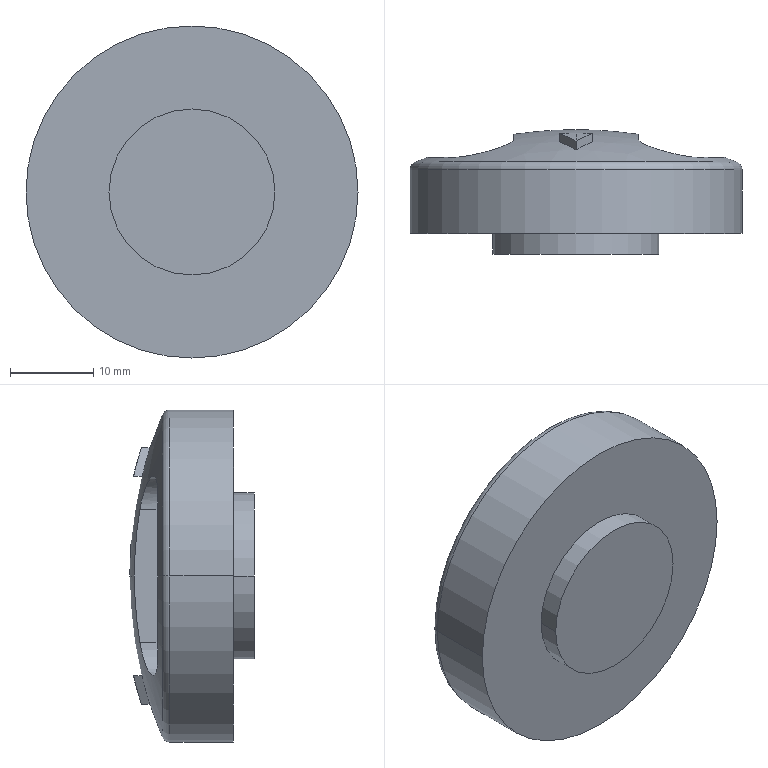Part | SolidWorks | features ICE 3, Fillet 1, RevCut 1, Revolution 1 | 1 solid | 31 faces | box 40 x 15 x 40 mm | volume 12868 mm3 | plane 12 | cylinder 11 | sphere 6 | torus 2 | commonest cylinder face diameters 7.99 x4 36 x3 20 x2 40 x2
STEP:
#1=CARTESIAN_POINT('',(-2.,12.028,-12.));
#2=VERTEX_POINT('',#1);
#3=CARTESIAN_POINT('',(0.,12.068,-12.));
#4=VERTEX_POINT('',#3);
#5=CARTESIAN_POINT('',(0.,-37.5,-12.));
#6=DIRECTION('',(0.,0.,-1.));
#7=DIRECTION('',(1.,0.,0.));
#8=AXIS2_PLACEMENT_3D('',#5,#6,#7);
#9=CIRCLE('',#8,49.568);
#10=EDGE_CURVE('',#2,#4,#9,.T.);
#11=ORIENTED_EDGE('',*,*,#10,.T.);
#12=CARTESIAN_POINT('',(0.,11.099,-15.464));
#13=VERTEX_POINT('',#12);
#14=CARTESIAN_POINT('',(0.,-37.5,0.));
#15=DIRECTION('',(-1.,0.,0.));
#16=DIRECTION('',(0.,0.,1.));
#17=AXIS2_PLACEMENT_3D('',#14,#15,#16);
#18=CIRCLE('',#17,51.);
#19=EDGE_CURVE('',#4,#13,#18,.T.);
#20=ORIENTED_EDGE('',*,*,#19,.T.);
#21=CARTESIAN_POINT('',(-6.696,-37.5,-3.866));
#22=DIRECTION('',(0.866,0.,0.5));
#23=DIRECTION('',(-0.5,0.,0.866));
#24=AXIS2_PLACEMENT_3D('',#21,#22,#23);
#25=CIRCLE('',#24,50.41);
#26=EDGE_CURVE('',#13,#2,#25,.T.);
#27=ORIENTED_EDGE('',*,*,#26,.T.);
#28=EDGE_LOOP('',(#11,#20,#27));
#29=FACE_OUTER_BOUND('',#28,.T.);
#30=CARTESIAN_POINT('',(0.,-37.5,0.));
#31=DIRECTION('',(1.,0.,0.));
#32=DIRECTION('',(0.,0.,-1.));
#33=AXIS2_PLACEMENT_3D('',#30,#31,#32);
#34=SPHERICAL_SURFACE('',#33,51.);
#35=ADVANCED_FACE('',(#29),#34,.T.);
#36=CARTESIAN_POINT('',(2.,12.028,12.));
#37=VERTEX_POINT('',#36);
#38=CARTESIAN_POINT('',(0.,12.068,12.));
#39=VERTEX_POINT('',#38);
#40=CARTESIAN_POINT('',(0.,-37.5,12.));
#41=DIRECTION('',(0.,0.,1.));
#42=DIRECTION('',(-1.,0.,0.));
#43=AXIS2_PLACEMENT_3D('',#40,#41,#42);
#44=CIRCLE('',#43,49.568);
#45=EDGE_CURVE('',#37,#39,#44,.T.);
#46=ORIENTED_EDGE('',*,*,#45,.T.);
#47=CARTESIAN_POINT('',(0.,11.099,15.464));
#48=VERTEX_POINT('',#47);
#49=CARTESIAN_POINT('',(0.,-37.5,0.));
#50=DIRECTION('',(1.,0.,0.));
#51=DIRECTION('',(0.,0.,-1.));
#52=AXIS2_PLACEMENT_3D('',#49,#50,#51);
#53=CIRCLE('',#52,51.);
#54=EDGE_CURVE('',#39,#48,#53,.T.);
#55=ORIENTED_EDGE('',*,*,#54,.T.);
#56=CARTESIAN_POINT('',(6.696,-37.5,3.866));
#57=DIRECTION('',(-0.866,0.,-0.5));
#58=DIRECTION('',(0.5,0.,-0.866));
#59=AXIS2_PLACEMENT_3D('',#56,#57,#58);
#60=CIRCLE('',#59,50.41);
#61=EDGE_CURVE('',#48,#37,#60,.T.);
#62=ORIENTED_EDGE('',*,*,#61,.T.);
#63=EDGE_LOOP('',(#46,#55,#62));
#64=FACE_OUTER_BOUND('',#63,.T.);
#65=CARTESIAN_POINT('',(0.,-37.5,0.));
#66=DIRECTION('',(1.,0.,0.));
#67=DIRECTION('',(0.,0.,-1.));
#68=AXIS2_PLACEMENT_3D('',#65,#66,#67);
#69=SPHERICAL_SURFACE('',#68,51.);
#70=ADVANCED_FACE('',(#64),#69,.T.);
#71=CARTESIAN_POINT('',(14.774,9.148,10.282));
#72=VERTEX_POINT('',#71);
#73=CARTESIAN_POINT('',(18.,9.148,0.));
#74=VERTEX_POINT('',#73);
#75=CARTESIAN_POINT('',(0.,9.148,0.));
#76=DIRECTION('',(0.,1.,0.));
#77=DIRECTION('',(1.,0.,0.));
#78=AXIS2_PLACEMENT_3D('',#75,#76,#77);
#79=CIRCLE('',#78,18.);
#80=EDGE_CURVE('',#72,#74,#79,.T.);
#81=ORIENTED_EDGE('',*,*,#80,.T.);
#82=CARTESIAN_POINT('',(18.,8.,0.));
#83=VERTEX_POINT('',#82);
#84=CARTESIAN_POINT('',(18.,18.5,0.));
#85=DIRECTION('',(0.,-1.,0.));
#86=VECTOR('',#85,1000.);
#87=LINE('',#84,#86);
#88=EDGE_CURVE('',#74,#83,#87,.T.);
#89=ORIENTED_EDGE('',*,*,#88,.T.);
#90=CARTESIAN_POINT('',(14.774,8.,10.282));
#91=VERTEX_POINT('',#90);
#92=CARTESIAN_POINT('',(0.,8.,0.));
#93=DIRECTION('',(0.,-1.,0.));
#94=DIRECTION('',(-1.,0.,0.));
#95=AXIS2_PLACEMENT_3D('',#92,#93,#94);
#96=CIRCLE('',#95,18.);
#97=EDGE_CURVE('',#83,#91,#96,.T.);
#98=ORIENTED_EDGE('',*,*,#97,.T.);
#99=CARTESIAN_POINT('',(14.774,18.5,10.282));
#100=DIRECTION('',(0.,-1.,0.));
#101=VECTOR('',#100,1000.);
#102=LINE('',#99,#101);
#103=EDGE_CURVE('',#72,#91,#102,.T.);
#104=ORIENTED_EDGE('',*,*,#103,.F.);
#105=EDGE_LOOP('',(#81,#89,#98,#104));
#106=FACE_OUTER_BOUND('',#105,.T.);
#107=CARTESIAN_POINT('',(0.,18.5,0.));
#108=DIRECTION('',(0.,-1.,0.));
#109=DIRECTION('',(1.,0.,0.));
#110=AXIS2_PLACEMENT_3D('',#107,#108,#109);
#111=CYLINDRICAL_SURFACE('',#110,18.);
#112=ADVANCED_FACE('',(#106),#111,.F.);
#113=CARTESIAN_POINT('',(10.,-2.5,0.));
#114=VERTEX_POINT('',#113);
#115=CARTESIAN_POINT('',(-10.,-2.5,0.));
#116=VERTEX_POINT('',#115);
#117=CARTESIAN_POINT('',(0.,-2.5,0.));
#118=DIRECTION('',(0.,-1.,0.));
#119=DIRECTION('',(1.,0.,0.));
#120=AXIS2_PLACEMENT_3D('',#117,#118,#119);
#121=CIRCLE('',#120,10.);
#122=EDGE_CURVE('',#114,#116,#121,.T.);
#123=ORIENTED_EDGE('',*,*,#122,.F.);
#124=CARTESIAN_POINT('',(10.,0.,0.));
#125=VERTEX_POINT('',#124);
#126=CARTESIAN_POINT('',(10.,-2.5,0.));
#127=DIRECTION('',(0.,1.,0.));
#128=VECTOR('',#127,1000.);
#129=LINE('',#126,#128);
#130=EDGE_CURVE('',#114,#125,#129,.T.);
#131=ORIENTED_EDGE('',*,*,#130,.T.);
#132=CARTESIAN_POINT('',(-10.,0.,0.));
#133=VERTEX_POINT('',#132);
#134=CARTESIAN_POINT('',(0.,0.,0.));
#135=DIRECTION('',(0.,-1.,0.));
#136=DIRECTION('',(1.,0.,0.));
#137=AXIS2_PLACEMENT_3D('',#134,#135,#136);
#138=CIRCLE('',#137,10.);
#139=EDGE_CURVE('',#125,#133,#138,.T.);
#140=ORIENTED_EDGE('',*,*,#139,.T.);
#141=CARTESIAN_POINT('',(-10.,-2.5,0.));
#142=DIRECTION('',(0.,1.,0.));
#143=VECTOR('',#142,1000.);
#144=LINE('',#141,#143);
#145=EDGE_CURVE('',#116,#133,#144,.T.);
#146=ORIENTED_EDGE('',*,*,#145,.F.);
#147=EDGE_LOOP('',(#123,#131,#140,#146));
#148=FACE_OUTER_BOUND('',#147,.T.);
#149=CARTESIAN_POINT('',(0.,-2.5,0.));
#150=DIRECTION('',(0.,1.,0.));
#151=DIRECTION('',(-1.,0.,0.));
#152=AXIS2_PLACEMENT_3D('',#149,#150,#151);
#153=CYLINDRICAL_SURFACE('',#152,10.);
#154=ADVANCED_FACE('',(#148),#153,.T.);
#155=CARTESIAN_POINT('',(-19.388,8.588,0.));
#156=VERTEX_POINT('',#155);
#157=CARTESIAN_POINT('',(19.388,8.588,0.));
#158=VERTEX_POINT('',#157);
#159=CARTESIAN_POINT('',(0.,8.588,0.));
#160=DIRECTION('',(0.,1.,0.));
#161=DIRECTION('',(1.,0.,0.));
#162=AXIS2_PLACEMENT_3D('',#159,#160,#161);
#163=CIRCLE('',#162,19.388);
#164=EDGE_CURVE('',#156,#158,#163,.T.);
#165=ORIENTED_EDGE('',*,*,#164,.F.);
#166=CARTESIAN_POINT('',(-20.,7.666,0.));
#167=VERTEX_POINT('',#166);
#168=CARTESIAN_POINT('',(-19.,7.666,0.));
#169=DIRECTION('',(0.,0.,1.));
#170=DIRECTION('',(1.,0.,0.));
#171=AXIS2_PLACEMENT_3D('',#168,#169,#170);
#172=CIRCLE('',#171,1.);
#173=EDGE_CURVE('',#156,#167,#172,.T.);
#174=ORIENTED_EDGE('',*,*,#173,.T.);
#175=CARTESIAN_POINT('',(20.,7.666,0.));
#176=VERTEX_POINT('',#175);
#177=CARTESIAN_POINT('',(0.,7.666,0.));
#178=DIRECTION('',(0.,-1.,0.));
#179=DIRECTION('',(1.,0.,0.));
#180=AXIS2_PLACEMENT_3D('',#177,#178,#179);
#181=CIRCLE('',#180,20.);
#182=EDGE_CURVE('',#176,#167,#181,.T.);
#183=ORIENTED_EDGE('',*,*,#182,.F.);
#184=CARTESIAN_POINT('',(19.,7.666,0.));
#185=DIRECTION('',(0.,0.,-1.));
#186=DIRECTION('',(-1.,0.,0.));
#187=AXIS2_PLACEMENT_3D('',#184,#185,#186);
#188=CIRCLE('',#187,1.);
#189=EDGE_CURVE('',#158,#176,#188,.T.);
#190=ORIENTED_EDGE('',*,*,#189,.F.);
#191=EDGE_LOOP('',(#165,#174,#183,#190));
#192=FACE_OUTER_BOUND('',#191,.T.);
#193=CARTESIAN_POINT('',(0.,7.666,0.));
#194=DIRECTION('',(0.,-1.,0.));
#195=DIRECTION('',(1.,0.,0.));
#196=AXIS2_PLACEMENT_3D('',#193,#194,#195);
#197=TOROIDAL_SURFACE('',#196,19.,1.);
#198=ADVANCED_FACE('',(#192),#197,.T.);
#199=ORIENTED_EDGE('',*,*,#182,.T.);
#200=CARTESIAN_POINT('',(-20.,0.,0.));
#201=VERTEX_POINT('',#200);
#202=CARTESIAN_POINT('',(-20.,0.,0.));
#203=DIRECTION('',(0.,-1.,0.));
#204=VECTOR('',#203,1000.);
#205=LINE('',#202,#204);
#206=EDGE_CURVE('',#167,#201,#205,.T.);
#207=ORIENTED_EDGE('',*,*,#206,.T.);
#208=CARTESIAN_POINT('',(20.,0.,0.));
#209=VERTEX_POINT('',#208);
#210=CARTESIAN_POINT('',(0.,0.,0.));
#211=DIRECTION('',(0.,-1.,0.));
#212=DIRECTION('',(1.,0.,0.));
#213=AXIS2_PLACEMENT_3D('',#210,#211,#212);
#214=CIRCLE('',#213,20.);
#215=EDGE_CURVE('',#209,#201,#214,.T.);
#216=ORIENTED_EDGE('',*,*,#215,.F.);
#217=CARTESIAN_POINT('',(20.,0.,0.));
#218=DIRECTION('',(0.,-1.,0.));
#219=VECTOR('',#218,1000.);
#220=LINE('',#217,#219);
#221=EDGE_CURVE('',#176,#209,#220,.T.);
#222=ORIENTED_EDGE('',*,*,#221,.F.);
#223=EDGE_LOOP('',(#199,#207,#216,#222));
#224=FACE_OUTER_BOUND('',#223,.T.);
#225=CARTESIAN_POINT('',(0.,0.,0.));
#226=DIRECTION('',(0.,-1.,0.));
#227=DIRECTION('',(1.,0.,0.));
#228=AXIS2_PLACEMENT_3D('',#225,#226,#227);
#229=CYLINDRICAL_SURFACE('',#228,20.);
#230=ADVANCED_FACE('',(#224),#229,.T.);
#231=CARTESIAN_POINT('',(2.,10.997,12.));
#232=VERTEX_POINT('',#231);
#233=CARTESIAN_POINT('',(-2.,10.997,12.));
#234=VERTEX_POINT('',#233);
#235=CARTESIAN_POINT('',(0.,-37.5,12.));
#236=DIRECTION('',(0.,0.,1.));
#237=DIRECTION('',(-1.,0.,0.));
#238=AXIS2_PLACEMENT_3D('',#235,#236,#237);
#239=CIRCLE('',#238,48.539);
#240=EDGE_CURVE('',#232,#234,#239,.T.);
#241=ORIENTED_EDGE('',*,*,#240,.F.);
#242=CARTESIAN_POINT('',(0.,10.049,15.464));
#243=VERTEX_POINT('',#242);
#244=CARTESIAN_POINT('',(6.696,-37.5,3.866));
#245=DIRECTION('',(-0.866,0.,-0.5));
#246=DIRECTION('',(0.5,0.,-0.866));
#247=AXIS2_PLACEMENT_3D('',#244,#245,#246);
#248=CIRCLE('',#247,49.399);
#249=EDGE_CURVE('',#243,#232,#248,.T.);
#250=ORIENTED_EDGE('',*,*,#249,.F.);
#251=CARTESIAN_POINT('',(-6.696,-37.5,3.866));
#252=DIRECTION('',(0.866,0.,-0.5));
#253=DIRECTION('',(0.5,0.,0.866));
#254=AXIS2_PLACEMENT_3D('',#251,#252,#253);
#255=CIRCLE('',#254,49.399);
#256=EDGE_CURVE('',#234,#243,#255,.T.);
#257=ORIENTED_EDGE('',*,*,#256,.F.);
#258=EDGE_LOOP('',(#241,#250,#257));
#259=FACE_BOUND('',#258,.T.);
#260=CARTESIAN_POINT('',(0.,12.5,0.));
#261=VERTEX_POINT('',#260);
#262=CARTESIAN_POINT('',(7.5,11.934,0.));
#263=VERTEX_POINT('',#262);
#264=CARTESIAN_POINT('',(0.,-37.5,0.));
#265=DIRECTION('',(0.,0.,-1.));
#266=DIRECTION('',(-1.,0.,0.));
#267=AXIS2_PLACEMENT_3D('',#264,#265,#266);
#268=CIRCLE('',#267,50.);
#269=EDGE_CURVE('',#261,#263,#268,.T.);
#270=ORIENTED_EDGE('',*,*,#269,.F.);
#271=CARTESIAN_POINT('',(-7.5,11.934,0.));
#272=VERTEX_POINT('',#271);
#273=CARTESIAN_POINT('',(0.,-37.5,0.));
#274=DIRECTION('',(0.,0.,1.));
#275=DIRECTION('',(1.,0.,0.));
#276=AXIS2_PLACEMENT_3D('',#273,#274,#275);
#277=CIRCLE('',#276,50.);
#278=EDGE_CURVE('',#261,#272,#277,.T.);
#279=ORIENTED_EDGE('',*,*,#278,.T.);
#280=CARTESIAN_POINT('',(-7.5,11.283,8.));
#281=VERTEX_POINT('',#280);
#282=CARTESIAN_POINT('',(-7.5,-37.5,0.));
#283=DIRECTION('',(-1.,0.,0.));
#284=DIRECTION('',(0.,0.,-1.));
#285=AXIS2_PLACEMENT_3D('',#282,#283,#284);
#286=CIRCLE('',#285,49.434);
#287=EDGE_CURVE('',#281,#272,#286,.T.);
#288=ORIENTED_EDGE('',*,*,#287,.F.);
#289=CARTESIAN_POINT('',(-14.774,9.148,10.282));
#290=VERTEX_POINT('',#289);
#291=CARTESIAN_POINT('',(-14.774,9.148,10.282));
#292=CARTESIAN_POINT('',(-14.525,9.148,10.64));
#293=CARTESIAN_POINT('',(-14.226,9.169,10.949));
#294=CARTESIAN_POINT('',(-13.528,9.251,11.466));
#295=CARTESIAN_POINT('',(-13.149,9.311,11.662));
#296=CARTESIAN_POINT('',(-12.334,9.465,11.93));
#297=CARTESIAN_POINT('',(-11.917,9.556,11.995));
#298=CARTESIAN_POINT('',(-11.071,9.762,11.995));
#299=CARTESIAN_POINT('',(-10.659,9.874,11.929));
#300=CARTESIAN_POINT('',(-10.063,10.051,11.736));
#301=CARTESIAN_POINT('',(-9.87,10.111,11.655));
#302=CARTESIAN_POINT('',(-9.501,10.231,11.468));
#303=CARTESIAN_POINT('',(-9.325,10.292,11.361));
#304=CARTESIAN_POINT('',(-8.988,10.413,11.118));
#305=CARTESIAN_POINT('',(-8.828,10.474,10.982));
#306=CARTESIAN_POINT('',(-8.534,10.593,10.69));
#307=CARTESIAN_POINT('',(-8.399,10.651,10.533));
#308=CARTESIAN_POINT('',(-8.153,10.766,10.198));
#309=CARTESIAN_POINT('',(-8.041,10.822,10.019));
#310=CARTESIAN_POINT('',(-7.849,10.929,9.646));
#311=CARTESIAN_POINT('',(-7.768,10.98,9.453));
#312=CARTESIAN_POINT('',(-7.571,11.125,8.857));
#313=CARTESIAN_POINT('',(-7.5,11.212,8.431));
#314=CARTESIAN_POINT('',(-7.5,11.283,8.));
#315=B_SPLINE_CURVE_WITH_KNOTS('',3,(#291,#292,#293,#294,#295,#296,#297,#298,#299,#300,#301,#302,#303,#304,#305,#306,#307,#308,#309,#310,#311,#312,#313,#314),.UNSPECIFIED.,.F.,.F.,(4,2,2,2,2,2,2,2,2,2,2,4),(0.000000345,0.001291,0.002581,0.003872,0.005162,0.005808,0.006453,0.007098,0.007744,0.008389,0.009034,0.01032),.UNSPECIFIED.);
#316=EDGE_CURVE('',#290,#281,#315,.T.);
#317=ORIENTED_EDGE('',*,*,#316,.F.);
#318=CARTESIAN_POINT('',(-18.,9.148,0.));
#319=VERTEX_POINT('',#318);
#320=CARTESIAN_POINT('',(0.,9.148,0.));
#321=DIRECTION('',(0.,1.,0.));
#322=DIRECTION('',(1.,0.,0.));
#323=AXIS2_PLACEMENT_3D('',#320,#321,#322);
#324=CIRCLE('',#323,18.);
#325=EDGE_CURVE('',#319,#290,#324,.T.);
#326=ORIENTED_EDGE('',*,*,#325,.F.);
#327=CARTESIAN_POINT('',(0.,-37.5,0.));
#328=DIRECTION('',(0.,0.,1.));
#329=DIRECTION('',(1.,0.,0.));
#330=AXIS2_PLACEMENT_3D('',#327,#328,#329);
#331=CIRCLE('',#330,50.);
#332=EDGE_CURVE('',#319,#156,#331,.T.);
#333=ORIENTED_EDGE('',*,*,#332,.T.);
#334=ORIENTED_EDGE('',*,*,#164,.T.);
#335=CARTESIAN_POINT('',(0.,-37.5,0.));
#336=DIRECTION('',(0.,0.,-1.));
#337=DIRECTION('',(-1.,0.,0.));
#338=AXIS2_PLACEMENT_3D('',#335,#336,#337);
#339=CIRCLE('',#338,50.);
#340=EDGE_CURVE('',#74,#158,#339,.T.);
#341=ORIENTED_EDGE('',*,*,#340,.F.);
#342=ORIENTED_EDGE('',*,*,#80,.F.);
#343=CARTESIAN_POINT('',(7.5,11.283,8.));
#344=VERTEX_POINT('',#343);
#345=CARTESIAN_POINT('',(7.5,11.283,8.));
#346=CARTESIAN_POINT('',(7.5,11.212,8.431));
#347=CARTESIAN_POINT('',(7.568,11.128,8.847));
#348=CARTESIAN_POINT('',(7.767,10.981,9.451));
#349=CARTESIAN_POINT('',(7.849,10.929,9.646));
#350=CARTESIAN_POINT('',(8.04,10.823,10.016));
#351=CARTESIAN_POINT('',(8.149,10.767,10.193));
#352=CARTESIAN_POINT('',(8.397,10.652,10.531));
#353=CARTESIAN_POINT('',(8.534,10.593,10.69));
#354=CARTESIAN_POINT('',(8.828,10.474,10.982));
#355=CARTESIAN_POINT('',(8.986,10.414,11.116));
#356=CARTESIAN_POINT('',(9.322,10.293,11.359));
#357=CARTESIAN_POINT('',(9.501,10.231,11.468));
#358=CARTESIAN_POINT('',(9.871,10.11,11.656));
#359=CARTESIAN_POINT('',(10.062,10.051,11.735));
#360=CARTESIAN_POINT('',(10.456,9.934,11.863));
#361=CARTESIAN_POINT('',(10.661,9.876,11.913));
#362=CARTESIAN_POINT('',(11.075,9.764,11.978));
#363=CARTESIAN_POINT('',(11.283,9.711,11.995));
#364=CARTESIAN_POINT('',(11.909,9.558,11.995));
#365=CARTESIAN_POINT('',(12.336,9.465,11.928));
#366=CARTESIAN_POINT('',(12.939,9.351,11.731));
#367=CARTESIAN_POINT('',(13.136,9.317,11.649));
#368=CARTESIAN_POINT('',(13.518,9.256,11.452));
#369=CARTESIAN_POINT('',(13.702,9.231,11.337));
#370=CARTESIAN_POINT('',(14.046,9.19,11.082));
#371=CARTESIAN_POINT('',(14.208,9.174,10.941));
#372=CARTESIAN_POINT('',(14.51,9.153,10.63));
#373=CARTESIAN_POINT('',(14.65,9.148,10.461));
#374=CARTESIAN_POINT('',(14.774,9.148,10.282));
#375=B_SPLINE_CURVE_WITH_KNOTS('',3,(#345,#346,#347,#348,#349,#350,#351,#352,#353,#354,#355,#356,#357,#358,#359,#360,#361,#362,#363,#364,#365,#366,#367,#368,#369,#370,#371,#372,#373,#374),.UNSPECIFIED.,.F.,.F.,(4,2,2,2,2,2,2,2,2,2,2,2,2,2,4),(0.0000002,0.001291,0.001936,0.002581,0.003226,0.003871,0.004516,0.005161,0.005807,0.006452,0.007742,0.008387,0.009032,0.009678,0.01032),.UNSPECIFIED.);
#376=EDGE_CURVE('',#344,#72,#375,.T.);
#377=ORIENTED_EDGE('',*,*,#376,.F.);
#378=CARTESIAN_POINT('',(7.5,-37.5,0.));
#379=DIRECTION('',(1.,0.,0.));
#380=DIRECTION('',(0.,0.,1.));
#381=AXIS2_PLACEMENT_3D('',#378,#379,#380);
#382=CIRCLE('',#381,49.434);
#383=EDGE_CURVE('',#263,#344,#382,.T.);
#384=ORIENTED_EDGE('',*,*,#383,.F.);
#385=EDGE_LOOP('',(#270,#279,#288,#317,#326,#333,#334,#341,#342,#377,#384));
#386=FACE_OUTER_BOUND('',#385,.T.);
#387=CARTESIAN_POINT('',(0.,-37.5,0.));
#388=DIRECTION('',(0.,0.,1.));
#389=DIRECTION('',(1.,0.,0.));
#390=AXIS2_PLACEMENT_3D('',#387,#388,#389);
#391=SPHERICAL_SURFACE('',#390,50.);
#392=ADVANCED_FACE('',(#259,#386),#391,.T.);
#393=ORIENTED_EDGE('',*,*,#10,.F.);
#394=CARTESIAN_POINT('',(-2.,10.997,-12.));
#395=VERTEX_POINT('',#394);
#396=CARTESIAN_POINT('',(-2.,13.5,-12.));
#397=DIRECTION('',(0.,-1.,0.));
#398=VECTOR('',#397,1000.);
#399=LINE('',#396,#398);
#400=EDGE_CURVE('',#2,#395,#399,.T.);
#401=ORIENTED_EDGE('',*,*,#400,.T.);
#402=CARTESIAN_POINT('',(2.,10.997,-12.));
#403=VERTEX_POINT('',#402);
#404=CARTESIAN_POINT('',(0.,-37.5,-12.));
#405=DIRECTION('',(0.,0.,-1.));
#406=DIRECTION('',(1.,0.,0.));
#407=AXIS2_PLACEMENT_3D('',#404,#405,#406);
#408=CIRCLE('',#407,48.539);
#409=EDGE_CURVE('',#395,#403,#408,.T.);
#410=ORIENTED_EDGE('',*,*,#409,.T.);
#411=CARTESIAN_POINT('',(2.,12.028,-12.));
#412=VERTEX_POINT('',#411);
#413=CARTESIAN_POINT('',(2.,13.5,-12.));
#414=DIRECTION('',(0.,-1.,0.));
#415=VECTOR('',#414,1000.);
#416=LINE('',#413,#415);
#417=EDGE_CURVE('',#412,#403,#416,.T.);
#418=ORIENTED_EDGE('',*,*,#417,.F.);
#419=CARTESIAN_POINT('',(0.,-37.5,-12.));
#420=DIRECTION('',(0.,0.,-1.));
#421=DIRECTION('',(1.,0.,0.));
#422=AXIS2_PLACEMENT_3D('',#419,#420,#421);
#423=CIRCLE('',#422,49.568);
#424=EDGE_CURVE('',#4,#412,#423,.T.);
#425=ORIENTED_EDGE('',*,*,#424,.F.);
#426=EDGE_LOOP('',(#393,#401,#410,#418,#425));
#427=FACE_OUTER_BOUND('',#426,.T.);
#428=CARTESIAN_POINT('',(-2.,13.5,-12.));
#429=DIRECTION('',(0.,0.,1.));
#430=DIRECTION('',(1.,0.,0.));
#431=AXIS2_PLACEMENT_3D('',#428,#429,#430);
#432=PLANE('',#431);
#433=ADVANCED_FACE('',(#427),#432,.T.);
#434=CARTESIAN_POINT('',(6.696,-37.5,-3.866));
#435=DIRECTION('',(-0.866,0.,0.5));
#436=DIRECTION('',(-0.5,0.,-0.866));
#437=AXIS2_PLACEMENT_3D('',#434,#435,#436);
#438=CIRCLE('',#437,50.41);
#439=EDGE_CURVE('',#412,#13,#438,.T.);
#440=ORIENTED_EDGE('',*,*,#439,.F.);
#441=ORIENTED_EDGE('',*,*,#417,.T.);
#442=CARTESIAN_POINT('',(0.,10.049,-15.464));
#443=VERTEX_POINT('',#442);
#444=CARTESIAN_POINT('',(6.696,-37.5,-3.866));
#445=DIRECTION('',(-0.866,0.,0.5));
#446=DIRECTION('',(-0.5,0.,-0.866));
#447=AXIS2_PLACEMENT_3D('',#444,#445,#446);
#448=CIRCLE('',#447,49.399);
#449=EDGE_CURVE('',#403,#443,#448,.T.);
#450=ORIENTED_EDGE('',*,*,#449,.T.);
#451=CARTESIAN_POINT('',(0.,13.5,-15.464));
#452=DIRECTION('',(0.,-1.,0.));
#453=VECTOR('',#452,1000.);
#454=LINE('',#451,#453);
#455=EDGE_CURVE('',#13,#443,#454,.T.);
#456=ORIENTED_EDGE('',*,*,#455,.F.);
#457=EDGE_LOOP('',(#440,#441,#450,#456));
#458=FACE_OUTER_BOUND('',#457,.T.);
#459=CARTESIAN_POINT('',(2.,13.5,-12.));
#460=DIRECTION('',(0.866,0.,-0.5));
#461=DIRECTION('',(-0.5,0.,-0.866));
#462=AXIS2_PLACEMENT_3D('',#459,#460,#461);
#463=PLANE('',#462);
#464=ADVANCED_FACE('',(#458),#463,.T.);
#465=ORIENTED_EDGE('',*,*,#26,.F.);
#466=ORIENTED_EDGE('',*,*,#455,.T.);
#467=CARTESIAN_POINT('',(-6.696,-37.5,-3.866));
#468=DIRECTION('',(0.866,0.,0.5));
#469=DIRECTION('',(-0.5,0.,0.866));
#470=AXIS2_PLACEMENT_3D('',#467,#468,#469);
#471=CIRCLE('',#470,49.399);
#472=EDGE_CURVE('',#443,#395,#471,.T.);
#473=ORIENTED_EDGE('',*,*,#472,.T.);
#474=ORIENTED_EDGE('',*,*,#400,.F.);
#475=EDGE_LOOP('',(#465,#466,#473,#474));
#476=FACE_OUTER_BOUND('',#475,.T.);
#477=CARTESIAN_POINT('',(0.,13.5,-15.464));
#478=DIRECTION('',(-0.866,0.,-0.5));
#479=DIRECTION('',(-0.5,0.,0.866));
#480=AXIS2_PLACEMENT_3D('',#477,#478,#479);
#481=PLANE('',#480);
#482=ADVANCED_FACE('',(#476),#481,.T.);
#483=ORIENTED_EDGE('',*,*,#45,.F.);
#484=CARTESIAN_POINT('',(2.,13.5,12.));
#485=DIRECTION('',(0.,-1.,0.));
#486=VECTOR('',#485,1000.);
#487=LINE('',#484,#486);
#488=EDGE_CURVE('',#37,#232,#487,.T.);
#489=ORIENTED_EDGE('',*,*,#488,.T.);
#490=ORIENTED_EDGE('',*,*,#240,.T.);
#491=CARTESIAN_POINT('',(-2.,12.028,12.));
#492=VERTEX_POINT('',#491);
#493=CARTESIAN_POINT('',(-2.,13.5,12.));
#494=DIRECTION('',(0.,-1.,0.));
#495=VECTOR('',#494,1000.);
#496=LINE('',#493,#495);
#497=EDGE_CURVE('',#492,#234,#496,.T.);
#498=ORIENTED_EDGE('',*,*,#497,.F.);
#499=CARTESIAN_POINT('',(0.,-37.5,12.));
#500=DIRECTION('',(0.,0.,1.));
#501=DIRECTION('',(-1.,0.,0.));
#502=AXIS2_PLACEMENT_3D('',#499,#500,#501);
#503=CIRCLE('',#502,49.568);
#504=EDGE_CURVE('',#39,#492,#503,.T.);
#505=ORIENTED_EDGE('',*,*,#504,.F.);
#506=EDGE_LOOP('',(#483,#489,#490,#498,#505));
#507=FACE_OUTER_BOUND('',#506,.T.);
#508=CARTESIAN_POINT('',(-2.,13.5,12.));
#509=DIRECTION('',(0.,0.,-1.));
#510=DIRECTION('',(-1.,0.,0.));
#511=AXIS2_PLACEMENT_3D('',#508,#509,#510);
#512=PLANE('',#511);
#513=ADVANCED_FACE('',(#507),#512,.T.);
#514=CARTESIAN_POINT('',(-6.696,-37.5,3.866));
#515=DIRECTION('',(0.866,0.,-0.5));
#516=DIRECTION('',(0.5,0.,0.866));
#517=AXIS2_PLACEMENT_3D('',#514,#515,#516);
#518=CIRCLE('',#517,50.41);
#519=EDGE_CURVE('',#492,#48,#518,.T.);
#520=ORIENTED_EDGE('',*,*,#519,.F.);
#521=ORIENTED_EDGE('',*,*,#497,.T.);
#522=ORIENTED_EDGE('',*,*,#256,.T.);
#523=CARTESIAN_POINT('',(0.,13.5,15.464));
#524=DIRECTION('',(0.,-1.,0.));
#525=VECTOR('',#524,1000.);
#526=LINE('',#523,#525);
#527=EDGE_CURVE('',#48,#243,#526,.T.);
#528=ORIENTED_EDGE('',*,*,#527,.F.);
#529=EDGE_LOOP('',(#520,#521,#522,#528));
#530=FACE_OUTER_BOUND('',#529,.T.);
#531=CARTESIAN_POINT('',(0.,13.5,15.464));
#532=DIRECTION('',(-0.866,0.,0.5));
#533=DIRECTION('',(0.5,0.,0.866));
#534=AXIS2_PLACEMENT_3D('',#531,#532,#533);
#535=PLANE('',#534);
#536=ADVANCED_FACE('',(#530),#535,.T.);
#537=ORIENTED_EDGE('',*,*,#61,.F.);
#538=ORIENTED_EDGE('',*,*,#527,.T.);
#539=ORIENTED_EDGE('',*,*,#249,.T.);
#540=ORIENTED_EDGE('',*,*,#488,.F.);
#541=EDGE_LOOP('',(#537,#538,#539,#540));
#542=FACE_OUTER_BOUND('',#541,.T.);
#543=CARTESIAN_POINT('',(2.,13.5,12.));
#544=DIRECTION('',(0.866,0.,0.5));
#545=DIRECTION('',(0.5,0.,-0.866));
#546=AXIS2_PLACEMENT_3D('',#543,#544,#545);
#547=PLANE('',#546);
#548=ADVANCED_FACE('',(#542),#547,.T.);
#549=ORIENTED_EDGE('',*,*,#278,.F.);
#550=ORIENTED_EDGE('',*,*,#269,.T.);
#551=CARTESIAN_POINT('',(7.5,11.283,-8.));
#552=VERTEX_POINT('',#551);
#553=CARTESIAN_POINT('',(7.5,-37.5,0.));
#554=DIRECTION('',(1.,0.,0.));
#555=DIRECTION('',(0.,0.,1.));
#556=AXIS2_PLACEMENT_3D('',#553,#554,#555);
#557=CIRCLE('',#556,49.434);
#558=EDGE_CURVE('',#552,#263,#557,.T.);
#559=ORIENTED_EDGE('',*,*,#558,.F.);
#560=CARTESIAN_POINT('',(14.774,9.148,-10.282));
#561=VERTEX_POINT('',#560);
#562=CARTESIAN_POINT('',(14.774,9.148,-10.282));
#563=CARTESIAN_POINT('',(14.525,9.148,-10.64));
#564=CARTESIAN_POINT('',(14.226,9.169,-10.949));
#565=CARTESIAN_POINT('',(13.528,9.251,-11.466));
#566=CARTESIAN_POINT('',(13.149,9.311,-11.662));
#567=CARTESIAN_POINT('',(12.334,9.465,-11.93));
#568=CARTESIAN_POINT('',(11.917,9.556,-11.995));
#569=CARTESIAN_POINT('',(11.071,9.762,-11.995));
#570=CARTESIAN_POINT('',(10.659,9.874,-11.929));
#571=CARTESIAN_POINT('',(10.063,10.051,-11.736));
#572=CARTESIAN_POINT('',(9.87,10.111,-11.655));
#573=CARTESIAN_POINT('',(9.501,10.231,-11.468));
#574=CARTESIAN_POINT('',(9.325,10.292,-11.361));
#575=CARTESIAN_POINT('',(8.988,10.413,-11.118));
#576=CARTESIAN_POINT('',(8.828,10.474,-10.982));
#577=CARTESIAN_POINT('',(8.534,10.593,-10.69));
#578=CARTESIAN_POINT('',(8.399,10.651,-10.533));
#579=CARTESIAN_POINT('',(8.153,10.766,-10.198));
#580=CARTESIAN_POINT('',(8.041,10.822,-10.019));
#581=CARTESIAN_POINT('',(7.849,10.929,-9.646));
#582=CARTESIAN_POINT('',(7.768,10.98,-9.453));
#583=CARTESIAN_POINT('',(7.571,11.125,-8.857));
#584=CARTESIAN_POINT('',(7.5,11.212,-8.431));
#585=CARTESIAN_POINT('',(7.5,11.283,-8.));
#586=B_SPLINE_CURVE_WITH_KNOTS('',3,(#562,#563,#564,#565,#566,#567,#568,#569,#570,#571,#572,#573,#574,#575,#576,#577,#578,#579,#580,#581,#582,#583,#584,#585),.UNSPECIFIED.,.F.,.F.,(4,2,2,2,2,2,2,2,2,2,2,4),(0.000000345,0.001291,0.002581,0.003872,0.005162,0.005808,0.006453,0.007098,0.007744,0.008389,0.009034,0.01032),.UNSPECIFIED.);
#587=EDGE_CURVE('',#561,#552,#586,.T.);
#588=ORIENTED_EDGE('',*,*,#587,.F.);
#589=CARTESIAN_POINT('',(0.,9.148,0.));
#590=DIRECTION('',(0.,1.,0.));
#591=DIRECTION('',(1.,0.,0.));
#592=AXIS2_PLACEMENT_3D('',#589,#590,#591);
#593=CIRCLE('',#592,18.);
#594=EDGE_CURVE('',#74,#561,#593,.T.);
#595=ORIENTED_EDGE('',*,*,#594,.F.);
#596=ORIENTED_EDGE('',*,*,#340,.T.);
#597=CARTESIAN_POINT('',(0.,8.588,0.));
#598=DIRECTION('',(0.,1.,0.));
#599=DIRECTION('',(1.,0.,0.));
#600=AXIS2_PLACEMENT_3D('',#597,#598,#599);
#601=CIRCLE('',#600,19.388);
#602=EDGE_CURVE('',#158,#156,#601,.T.);
#603=ORIENTED_EDGE('',*,*,#602,.T.);
#604=ORIENTED_EDGE('',*,*,#332,.F.);
#605=CARTESIAN_POINT('',(-14.774,9.148,-10.282));
#606=VERTEX_POINT('',#605);
#607=CARTESIAN_POINT('',(0.,9.148,0.));
#608=DIRECTION('',(0.,1.,0.));
#609=DIRECTION('',(1.,0.,0.));
#610=AXIS2_PLACEMENT_3D('',#607,#608,#609);
#611=CIRCLE('',#610,18.);
#612=EDGE_CURVE('',#606,#319,#611,.T.);
#613=ORIENTED_EDGE('',*,*,#612,.F.);
#614=CARTESIAN_POINT('',(-7.5,11.283,-8.));
#615=VERTEX_POINT('',#614);
#616=CARTESIAN_POINT('',(-7.5,11.283,-8.));
#617=CARTESIAN_POINT('',(-7.5,11.212,-8.431));
#618=CARTESIAN_POINT('',(-7.568,11.128,-8.847));
#619=CARTESIAN_POINT('',(-7.767,10.981,-9.451));
#620=CARTESIAN_POINT('',(-7.849,10.929,-9.646));
#621=CARTESIAN_POINT('',(-8.04,10.823,-10.016));
#622=CARTESIAN_POINT('',(-8.149,10.767,-10.193));
#623=CARTESIAN_POINT('',(-8.397,10.652,-10.531));
#624=CARTESIAN_POINT('',(-8.534,10.593,-10.69));
#625=CARTESIAN_POINT('',(-8.828,10.474,-10.982));
#626=CARTESIAN_POINT('',(-8.986,10.414,-11.116));
#627=CARTESIAN_POINT('',(-9.322,10.293,-11.359));
#628=CARTESIAN_POINT('',(-9.501,10.231,-11.468));
#629=CARTESIAN_POINT('',(-9.871,10.11,-11.656));
#630=CARTESIAN_POINT('',(-10.062,10.051,-11.735));
#631=CARTESIAN_POINT('',(-10.456,9.934,-11.863));
#632=CARTESIAN_POINT('',(-10.661,9.876,-11.913));
#633=CARTESIAN_POINT('',(-11.075,9.764,-11.978));
#634=CARTESIAN_POINT('',(-11.283,9.711,-11.995));
#635=CARTESIAN_POINT('',(-11.909,9.558,-11.995));
#636=CARTESIAN_POINT('',(-12.336,9.465,-11.928));
#637=CARTESIAN_POINT('',(-12.939,9.351,-11.731));
#638=CARTESIAN_POINT('',(-13.136,9.317,-11.649));
#639=CARTESIAN_POINT('',(-13.518,9.256,-11.452));
#640=CARTESIAN_POINT('',(-13.702,9.231,-11.337));
#641=CARTESIAN_POINT('',(-14.046,9.19,-11.082));
#642=CARTESIAN_POINT('',(-14.208,9.174,-10.941));
#643=CARTESIAN_POINT('',(-14.51,9.153,-10.63));
#644=CARTESIAN_POINT('',(-14.65,9.148,-10.461));
#645=CARTESIAN_POINT('',(-14.774,9.148,-10.282));
#646=B_SPLINE_CURVE_WITH_KNOTS('',3,(#616,#617,#618,#619,#620,#621,#622,#623,#624,#625,#626,#627,#628,#629,#630,#631,#632,#633,#634,#635,#636,#637,#638,#639,#640,#641,#642,#643,#644,#645),.UNSPECIFIED.,.F.,.F.,(4,2,2,2,2,2,2,2,2,2,2,2,2,2,4),(0.0000002,0.001291,0.001936,0.002581,0.003226,0.003871,0.004516,0.005161,0.005807,0.006452,0.007742,0.008387,0.009032,0.009678,0.01032),.UNSPECIFIED.);
#647=EDGE_CURVE('',#615,#606,#646,.T.);
#648=ORIENTED_EDGE('',*,*,#647,.F.);
#649=CARTESIAN_POINT('',(-7.5,-37.5,0.));
#650=DIRECTION('',(-1.,0.,0.));
#651=DIRECTION('',(0.,0.,-1.));
#652=AXIS2_PLACEMENT_3D('',#649,#650,#651);
#653=CIRCLE('',#652,49.434);
#654=EDGE_CURVE('',#272,#615,#653,.T.);
#655=ORIENTED_EDGE('',*,*,#654,.F.);
#656=EDGE_LOOP('',(#549,#550,#559,#588,#595,#596,#603,#604,#613,#648,#655));
#657=FACE_OUTER_BOUND('',#656,.T.);
#658=ORIENTED_EDGE('',*,*,#409,.F.);
#659=ORIENTED_EDGE('',*,*,#472,.F.);
#660=ORIENTED_EDGE('',*,*,#449,.F.);
#661=EDGE_LOOP('',(#658,#659,#660));
#662=FACE_BOUND('',#661,.T.);
#663=CARTESIAN_POINT('',(0.,-37.5,0.));
#664=DIRECTION('',(0.,0.,1.));
#665=DIRECTION('',(1.,0.,0.));
#666=AXIS2_PLACEMENT_3D('',#663,#664,#665);
#667=SPHERICAL_SURFACE('',#666,50.);
#668=ADVANCED_FACE('',(#657,#662),#667,.T.);
#669=ORIENTED_EDGE('',*,*,#206,.F.);
#670=CARTESIAN_POINT('',(0.,7.666,0.));
#671=DIRECTION('',(0.,-1.,0.));
#672=DIRECTION('',(1.,0.,0.));
#673=AXIS2_PLACEMENT_3D('',#670,#671,#672);
#674=CIRCLE('',#673,20.);
#675=EDGE_CURVE('',#167,#176,#674,.T.);
#676=ORIENTED_EDGE('',*,*,#675,.T.);
#677=ORIENTED_EDGE('',*,*,#221,.T.);
#678=CARTESIAN_POINT('',(0.,0.,0.));
#679=DIRECTION('',(0.,-1.,0.));
#680=DIRECTION('',(1.,0.,0.));
#681=AXIS2_PLACEMENT_3D('',#678,#679,#680);
#682=CIRCLE('',#681,20.);
#683=EDGE_CURVE('',#201,#209,#682,.T.);
#684=ORIENTED_EDGE('',*,*,#683,.F.);
#685=EDGE_LOOP('',(#669,#676,#677,#684));
#686=FACE_OUTER_BOUND('',#685,.T.);
#687=CARTESIAN_POINT('',(0.,0.,0.));
#688=DIRECTION('',(0.,-1.,0.));
#689=DIRECTION('',(1.,0.,0.));
#690=AXIS2_PLACEMENT_3D('',#687,#688,#689);
#691=CYLINDRICAL_SURFACE('',#690,20.);
#692=ADVANCED_FACE('',(#686),#691,.T.);
#693=CARTESIAN_POINT('',(0.,0.,0.));
#694=DIRECTION('',(0.,-1.,0.));
#695=DIRECTION('',(1.,0.,0.));
#696=AXIS2_PLACEMENT_3D('',#693,#694,#695);
#697=CIRCLE('',#696,10.);
#698=EDGE_CURVE('',#133,#125,#697,.T.);
#699=ORIENTED_EDGE('',*,*,#698,.F.);
#700=ORIENTED_EDGE('',*,*,#139,.F.);
#701=EDGE_LOOP('',(#699,#700));
#702=FACE_BOUND('',#701,.T.);
#703=ORIENTED_EDGE('',*,*,#215,.T.);
#704=ORIENTED_EDGE('',*,*,#683,.T.);
#705=EDGE_LOOP('',(#703,#704));
#706=FACE_OUTER_BOUND('',#705,.T.);
#707=CARTESIAN_POINT('',(20.,0.,0.));
#708=DIRECTION('',(0.,-1.,0.));
#709=DIRECTION('',(1.,0.,0.));
#710=AXIS2_PLACEMENT_3D('',#707,#708,#709);
#711=PLANE('',#710);
#712=ADVANCED_FACE('',(#702,#706),#711,.T.);
#713=ORIENTED_EDGE('',*,*,#173,.F.);
#714=ORIENTED_EDGE('',*,*,#602,.F.);
#715=ORIENTED_EDGE('',*,*,#189,.T.);
#716=ORIENTED_EDGE('',*,*,#675,.F.);
#717=EDGE_LOOP('',(#713,#714,#715,#716));
#718=FACE_OUTER_BOUND('',#717,.T.);
#719=CARTESIAN_POINT('',(0.,7.666,0.));
#720=DIRECTION('',(0.,-1.,0.));
#721=DIRECTION('',(1.,0.,0.));
#722=AXIS2_PLACEMENT_3D('',#719,#720,#721);
#723=TOROIDAL_SURFACE('',#722,19.,1.);
#724=ADVANCED_FACE('',(#718),#723,.T.);
#725=ORIENTED_EDGE('',*,*,#130,.F.);
#726=CARTESIAN_POINT('',(0.,-2.5,0.));
#727=DIRECTION('',(0.,-1.,0.));
#728=DIRECTION('',(1.,0.,0.));
#729=AXIS2_PLACEMENT_3D('',#726,#727,#728);
#730=CIRCLE('',#729,10.);
#731=EDGE_CURVE('',#116,#114,#730,.T.);
#732=ORIENTED_EDGE('',*,*,#731,.F.);
#733=ORIENTED_EDGE('',*,*,#145,.T.);
#734=ORIENTED_EDGE('',*,*,#698,.T.);
#735=EDGE_LOOP('',(#725,#732,#733,#734));
#736=FACE_OUTER_BOUND('',#735,.T.);
#737=CARTESIAN_POINT('',(0.,-2.5,0.));
#738=DIRECTION('',(0.,1.,0.));
#739=DIRECTION('',(-1.,0.,0.));
#740=AXIS2_PLACEMENT_3D('',#737,#738,#739);
#741=CYLINDRICAL_SURFACE('',#740,10.);
#742=ADVANCED_FACE('',(#736),#741,.T.);
#743=ORIENTED_EDGE('',*,*,#731,.T.);
#744=ORIENTED_EDGE('',*,*,#122,.T.);
#745=EDGE_LOOP('',(#743,#744));
#746=FACE_OUTER_BOUND('',#745,.T.);
#747=CARTESIAN_POINT('',(0.,-2.5,0.));
#748=DIRECTION('',(0.,-1.,0.));
#749=DIRECTION('',(1.,0.,0.));
#750=AXIS2_PLACEMENT_3D('',#747,#748,#749);
#751=PLANE('',#750);
#752=ADVANCED_FACE('',(#746),#751,.T.);
#753=ORIENTED_EDGE('',*,*,#376,.T.);
#754=ORIENTED_EDGE('',*,*,#103,.T.);
#755=CARTESIAN_POINT('',(7.5,8.,8.));
#756=VERTEX_POINT('',#755);
#757=CARTESIAN_POINT('',(11.495,8.,8.));
#758=DIRECTION('',(0.,-1.,0.));
#759=DIRECTION('',(-1.,0.,0.));
#760=AXIS2_PLACEMENT_3D('',#757,#758,#759);
#761=CIRCLE('',#760,3.995);
#762=EDGE_CURVE('',#91,#756,#761,.T.);
#763=ORIENTED_EDGE('',*,*,#762,.T.);
#764=CARTESIAN_POINT('',(7.5,18.5,8.));
#765=DIRECTION('',(0.,-1.,0.));
#766=VECTOR('',#765,1000.);
#767=LINE('',#764,#766);
#768=EDGE_CURVE('',#344,#756,#767,.T.);
#769=ORIENTED_EDGE('',*,*,#768,.F.);
#770=EDGE_LOOP('',(#753,#754,#763,#769));
#771=FACE_OUTER_BOUND('',#770,.T.);
#772=CARTESIAN_POINT('',(11.495,18.5,8.));
#773=DIRECTION('',(0.,-1.,0.));
#774=DIRECTION('',(1.,0.,0.));
#775=AXIS2_PLACEMENT_3D('',#772,#773,#774);
#776=CYLINDRICAL_SURFACE('',#775,3.995);
#777=ADVANCED_FACE('',(#771),#776,.F.);
#778=ORIENTED_EDGE('',*,*,#88,.F.);
#779=ORIENTED_EDGE('',*,*,#594,.T.);
#780=CARTESIAN_POINT('',(14.774,8.,-10.282));
#781=VERTEX_POINT('',#780);
#782=CARTESIAN_POINT('',(14.774,18.5,-10.282));
#783=DIRECTION('',(0.,-1.,0.));
#784=VECTOR('',#783,1000.);
#785=LINE('',#782,#784);
#786=EDGE_CURVE('',#561,#781,#785,.T.);
#787=ORIENTED_EDGE('',*,*,#786,.T.);
#788=CARTESIAN_POINT('',(0.,8.,0.));
#789=DIRECTION('',(0.,-1.,0.));
#790=DIRECTION('',(-1.,0.,0.));
#791=AXIS2_PLACEMENT_3D('',#788,#789,#790);
#792=CIRCLE('',#791,18.);
#793=EDGE_CURVE('',#781,#83,#792,.T.);
#794=ORIENTED_EDGE('',*,*,#793,.T.);
#795=EDGE_LOOP('',(#778,#779,#787,#794));
#796=FACE_OUTER_BOUND('',#795,.T.);
#797=CARTESIAN_POINT('',(0.,18.5,0.));
#798=DIRECTION('',(0.,-1.,0.));
#799=DIRECTION('',(1.,0.,0.));
#800=AXIS2_PLACEMENT_3D('',#797,#798,#799);
#801=CYLINDRICAL_SURFACE('',#800,18.);
#802=ADVANCED_FACE('',(#796),#801,.F.);
#803=ORIENTED_EDGE('',*,*,#587,.T.);
#804=CARTESIAN_POINT('',(7.5,8.,-8.));
#805=VERTEX_POINT('',#804);
#806=CARTESIAN_POINT('',(7.5,18.5,-8.));
#807=DIRECTION('',(0.,-1.,0.));
#808=VECTOR('',#807,1000.);
#809=LINE('',#806,#808);
#810=EDGE_CURVE('',#552,#805,#809,.T.);
#811=ORIENTED_EDGE('',*,*,#810,.T.);
#812=CARTESIAN_POINT('',(11.495,8.,-8.));
#813=DIRECTION('',(0.,-1.,0.));
#814=DIRECTION('',(-1.,0.,0.));
#815=AXIS2_PLACEMENT_3D('',#812,#813,#814);
#816=CIRCLE('',#815,3.995);
#817=EDGE_CURVE('',#805,#781,#816,.T.);
#818=ORIENTED_EDGE('',*,*,#817,.T.);
#819=ORIENTED_EDGE('',*,*,#786,.F.);
#820=EDGE_LOOP('',(#803,#811,#818,#819));
#821=FACE_OUTER_BOUND('',#820,.T.);
#822=CARTESIAN_POINT('',(11.495,18.5,-8.));
#823=DIRECTION('',(0.,-1.,0.));
#824=DIRECTION('',(1.,0.,0.));
#825=AXIS2_PLACEMENT_3D('',#822,#823,#824);
#826=CYLINDRICAL_SURFACE('',#825,3.995);
#827=ADVANCED_FACE('',(#821),#826,.F.);
#828=ORIENTED_EDGE('',*,*,#558,.T.);
#829=ORIENTED_EDGE('',*,*,#383,.T.);
#830=ORIENTED_EDGE('',*,*,#768,.T.);
#831=CARTESIAN_POINT('',(7.5,8.,-8.));
#832=DIRECTION('',(0.,0.,-1.));
#833=VECTOR('',#832,1000.);
#834=LINE('',#831,#833);
#835=EDGE_CURVE('',#756,#805,#834,.T.);
#836=ORIENTED_EDGE('',*,*,#835,.T.);
#837=ORIENTED_EDGE('',*,*,#810,.F.);
#838=EDGE_LOOP('',(#828,#829,#830,#836,#837));
#839=FACE_OUTER_BOUND('',#838,.T.);
#840=CARTESIAN_POINT('',(7.5,18.5,-8.));
#841=DIRECTION('',(-1.,0.,0.));
#842=DIRECTION('',(0.,0.,1.));
#843=AXIS2_PLACEMENT_3D('',#840,#841,#842);
#844=PLANE('',#843);
#845=ADVANCED_FACE('',(#839),#844,.F.);
#846=ORIENTED_EDGE('',*,*,#762,.F.);
#847=ORIENTED_EDGE('',*,*,#97,.F.);
#848=ORIENTED_EDGE('',*,*,#793,.F.);
#849=ORIENTED_EDGE('',*,*,#817,.F.);
#850=ORIENTED_EDGE('',*,*,#835,.F.);
#851=EDGE_LOOP('',(#846,#847,#848,#849,#850));
#852=FACE_OUTER_BOUND('',#851,.T.);
#853=CARTESIAN_POINT('',(11.495,8.,8.));
#854=DIRECTION('',(0.,1.,0.));
#855=DIRECTION('',(-1.,0.,0.));
#856=AXIS2_PLACEMENT_3D('',#853,#854,#855);
#857=PLANE('',#856);
#858=ADVANCED_FACE('',(#852),#857,.T.);
#859=ORIENTED_EDGE('',*,*,#647,.T.);
#860=CARTESIAN_POINT('',(-14.774,8.,-10.282));
#861=VERTEX_POINT('',#860);
#862=CARTESIAN_POINT('',(-14.774,18.5,-10.282));
#863=DIRECTION('',(0.,-1.,0.));
#864=VECTOR('',#863,1000.);
#865=LINE('',#862,#864);
#866=EDGE_CURVE('',#606,#861,#865,.T.);
#867=ORIENTED_EDGE('',*,*,#866,.T.);
#868=CARTESIAN_POINT('',(-7.5,8.,-8.));
#869=VERTEX_POINT('',#868);
#870=CARTESIAN_POINT('',(-11.495,8.,-8.));
#871=DIRECTION('',(0.,-1.,0.));
#872=DIRECTION('',(1.,0.,0.));
#873=AXIS2_PLACEMENT_3D('',#870,#871,#872);
#874=CIRCLE('',#873,3.995);
#875=EDGE_CURVE('',#861,#869,#874,.T.);
#876=ORIENTED_EDGE('',*,*,#875,.T.);
#877=CARTESIAN_POINT('',(-7.5,18.5,-8.));
#878=DIRECTION('',(0.,-1.,0.));
#879=VECTOR('',#878,1000.);
#880=LINE('',#877,#879);
#881=EDGE_CURVE('',#615,#869,#880,.T.);
#882=ORIENTED_EDGE('',*,*,#881,.F.);
#883=EDGE_LOOP('',(#859,#867,#876,#882));
#884=FACE_OUTER_BOUND('',#883,.T.);
#885=CARTESIAN_POINT('',(-11.495,18.5,-8.));
#886=DIRECTION('',(0.,-1.,0.));
#887=DIRECTION('',(1.,0.,0.));
#888=AXIS2_PLACEMENT_3D('',#885,#886,#887);
#889=CYLINDRICAL_SURFACE('',#888,3.995);
#890=ADVANCED_FACE('',(#884),#889,.F.);
#891=ORIENTED_EDGE('',*,*,#612,.T.);
#892=ORIENTED_EDGE('',*,*,#325,.T.);
#893=CARTESIAN_POINT('',(-14.774,8.,10.282));
#894=VERTEX_POINT('',#893);
#895=CARTESIAN_POINT('',(-14.774,18.5,10.282));
#896=DIRECTION('',(0.,-1.,0.));
#897=VECTOR('',#896,1000.);
#898=LINE('',#895,#897);
#899=EDGE_CURVE('',#290,#894,#898,.T.);
#900=ORIENTED_EDGE('',*,*,#899,.T.);
#901=CARTESIAN_POINT('',(0.,8.,0.));
#902=DIRECTION('',(0.,-1.,0.));
#903=DIRECTION('',(1.,0.,0.));
#904=AXIS2_PLACEMENT_3D('',#901,#902,#903);
#905=CIRCLE('',#904,18.);
#906=EDGE_CURVE('',#894,#861,#905,.T.);
#907=ORIENTED_EDGE('',*,*,#906,.T.);
#908=ORIENTED_EDGE('',*,*,#866,.F.);
#909=EDGE_LOOP('',(#891,#892,#900,#907,#908));
#910=FACE_OUTER_BOUND('',#909,.T.);
#911=CARTESIAN_POINT('',(0.,18.5,0.));
#912=DIRECTION('',(0.,-1.,0.));
#913=DIRECTION('',(1.,0.,0.));
#914=AXIS2_PLACEMENT_3D('',#911,#912,#913);
#915=CYLINDRICAL_SURFACE('',#914,18.);
#916=ADVANCED_FACE('',(#910),#915,.F.);
#917=ORIENTED_EDGE('',*,*,#316,.T.);
#918=CARTESIAN_POINT('',(-7.5,8.,8.));
#919=VERTEX_POINT('',#918);
#920=CARTESIAN_POINT('',(-7.5,18.5,8.));
#921=DIRECTION('',(0.,-1.,0.));
#922=VECTOR('',#921,1000.);
#923=LINE('',#920,#922);
#924=EDGE_CURVE('',#281,#919,#923,.T.);
#925=ORIENTED_EDGE('',*,*,#924,.T.);
#926=CARTESIAN_POINT('',(-11.495,8.,8.));
#927=DIRECTION('',(0.,-1.,0.));
#928=DIRECTION('',(1.,0.,0.));
#929=AXIS2_PLACEMENT_3D('',#926,#927,#928);
#930=CIRCLE('',#929,3.995);
#931=EDGE_CURVE('',#919,#894,#930,.T.);
#932=ORIENTED_EDGE('',*,*,#931,.T.);
#933=ORIENTED_EDGE('',*,*,#899,.F.);
#934=EDGE_LOOP('',(#917,#925,#932,#933));
#935=FACE_OUTER_BOUND('',#934,.T.);
#936=CARTESIAN_POINT('',(-11.495,18.5,8.));
#937=DIRECTION('',(0.,-1.,0.));
#938=DIRECTION('',(1.,0.,0.));
#939=AXIS2_PLACEMENT_3D('',#936,#937,#938);
#940=CYLINDRICAL_SURFACE('',#939,3.995);
#941=ADVANCED_FACE('',(#935),#940,.F.);
#942=ORIENTED_EDGE('',*,*,#287,.T.);
#943=ORIENTED_EDGE('',*,*,#654,.T.);
#944=ORIENTED_EDGE('',*,*,#881,.T.);
#945=CARTESIAN_POINT('',(-7.5,8.,-8.));
#946=DIRECTION('',(0.,0.,1.));
#947=VECTOR('',#946,1000.);
#948=LINE('',#945,#947);
#949=EDGE_CURVE('',#869,#919,#948,.T.);
#950=ORIENTED_EDGE('',*,*,#949,.T.);
#951=ORIENTED_EDGE('',*,*,#924,.F.);
#952=EDGE_LOOP('',(#942,#943,#944,#950,#951));
#953=FACE_OUTER_BOUND('',#952,.T.);
#954=CARTESIAN_POINT('',(-7.5,18.5,-8.));
#955=DIRECTION('',(1.,0.,0.));
#956=DIRECTION('',(0.,0.,-1.));
#957=AXIS2_PLACEMENT_3D('',#954,#955,#956);
#958=PLANE('',#957);
#959=ADVANCED_FACE('',(#953),#958,.F.);
#960=ORIENTED_EDGE('',*,*,#875,.F.);
#961=ORIENTED_EDGE('',*,*,#906,.F.);
#962=ORIENTED_EDGE('',*,*,#931,.F.);
#963=ORIENTED_EDGE('',*,*,#949,.F.);
#964=EDGE_LOOP('',(#960,#961,#962,#963));
#965=FACE_OUTER_BOUND('',#964,.T.);
#966=CARTESIAN_POINT('',(-11.495,8.,-8.));
#967=DIRECTION('',(0.,-1.,0.));
#968=DIRECTION('',(1.,0.,0.));
#969=AXIS2_PLACEMENT_3D('',#966,#967,#968);
#970=PLANE('',#969);
#971=ADVANCED_FACE('',(#965),#970,.F.);
#972=ORIENTED_EDGE('',*,*,#54,.F.);
#973=ORIENTED_EDGE('',*,*,#504,.T.);
#974=ORIENTED_EDGE('',*,*,#519,.T.);
#975=EDGE_LOOP('',(#972,#973,#974));
#976=FACE_OUTER_BOUND('',#975,.T.);
#977=CARTESIAN_POINT('',(0.,-37.5,0.));
#978=DIRECTION('',(1.,0.,0.));
#979=DIRECTION('',(0.,0.,-1.));
#980=AXIS2_PLACEMENT_3D('',#977,#978,#979);
#981=SPHERICAL_SURFACE('',#980,51.);
#982=ADVANCED_FACE('',(#976),#981,.T.);
#983=ORIENTED_EDGE('',*,*,#19,.F.);
#984=ORIENTED_EDGE('',*,*,#424,.T.);
#985=ORIENTED_EDGE('',*,*,#439,.T.);
#986=EDGE_LOOP('',(#983,#984,#985));
#987=FACE_OUTER_BOUND('',#986,.T.);
#988=CARTESIAN_POINT('',(0.,-37.5,0.));
#989=DIRECTION('',(1.,0.,0.));
#990=DIRECTION('',(0.,0.,-1.));
#991=AXIS2_PLACEMENT_3D('',#988,#989,#990);
#992=SPHERICAL_SURFACE('',#991,51.);
#993=ADVANCED_FACE('',(#987),#992,.T.);
#994=CLOSED_SHELL('',(#35,#70,#112,#154,#198,#230,#392,#433,#464,#482,#513,#536,#548,#668,#692,#712,#724,#742,#752,#777,#802,#827,#845,#858,#890,#916,#941,#959,#971,#982,#993));
#995=MANIFOLD_SOLID_BREP('',#994);
#996=CARTESIAN_POINT('',(0.,0.,0.));
#997=DIRECTION('',(0.,0.,1.));
#998=DIRECTION('',(1.,0.,0.));
#999=AXIS2_PLACEMENT_3D('',#996,#997,#998);
#1000=(LENGTH_UNIT()NAMED_UNIT(*)SI_UNIT(.MILLI.,.METRE.));
#1001=UNCERTAINTY_MEASURE_WITH_UNIT(LENGTH_MEASURE(0.00001),#1000,'','');
#1002=(NAMED_UNIT(*)PLANE_ANGLE_UNIT()SI_UNIT($,.RADIAN.));
#1003=(NAMED_UNIT(*)SI_UNIT($,.STERADIAN.)SOLID_ANGLE_UNIT());
#1004=(GEOMETRIC_REPRESENTATION_CONTEXT(3)GLOBAL_UNCERTAINTY_ASSIGNED_CONTEXT((#1001))GLOBAL_UNIT_ASSIGNED_CONTEXT((#1000,#1002,#1003))REPRESENTATION_CONTEXT('',''));
#1005=ADVANCED_BREP_SHAPE_REPRESENTATION('',(#995,#999),#1004);